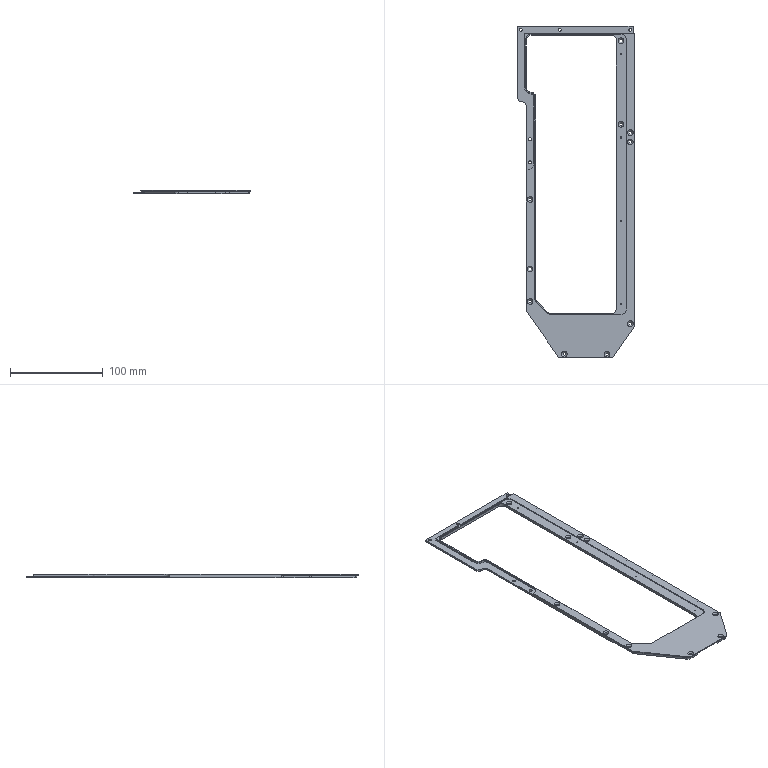NC program | NX | posted with a generic post | part box 127 x 358 x 4 mm
Whole program:
N10 G17 G21 G94 G90
(SPOT_DRILL_COPY_1_COPY , TOOL : CHAMFER_D8-90DEG)
N12 T01 M6
N14 G54
N16 G17 G0 G90 X-175. Y12.5 S2500 M3
N18 G43 Z5. H1
N20 G94 G82 G98 Z-2.6 F250. P200 R3.
N22 Y-33.5
N24 G80
N26 G0 X-175. Y-33.5 Z5.
N28 M5
N30 M2